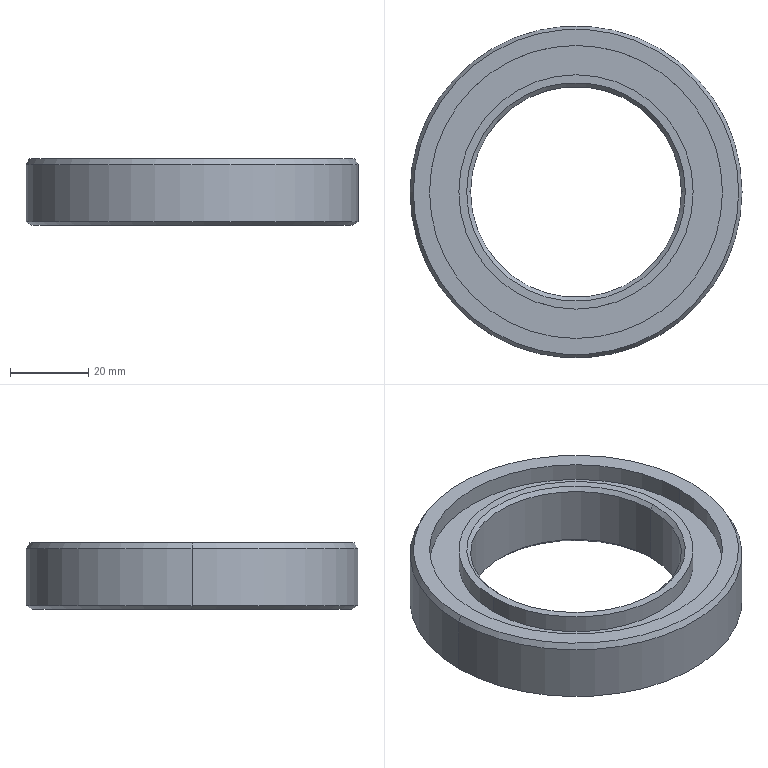Part | SolidWorks | features Chamfer 2, ICE 2, Extrusion 1 | 1 solid | 26 faces | box 85 x 85 x 17 mm | volume 42385 mm3 | cylinder 12 | cone 8 | plane 6 | commonest cylinder face diameters 60 x4 75 x4 54 x2 85 x2
STEP:
#1=CARTESIAN_POINT('',(-27.,0.,16.));
#2=VERTEX_POINT('',#1);
#3=CARTESIAN_POINT('',(27.,0.,16.));
#4=VERTEX_POINT('',#3);
#5=CARTESIAN_POINT('',(0.,0.,16.));
#6=DIRECTION('',(0.,0.,1.));
#7=DIRECTION('',(1.,0.,0.));
#8=AXIS2_PLACEMENT_3D('',#5,#6,#7);
#9=CIRCLE('',#8,27.);
#10=EDGE_CURVE('',#2,#4,#9,.T.);
#11=ORIENTED_EDGE('',*,*,#10,.F.);
#12=CARTESIAN_POINT('',(-28.,0.,17.));
#13=VERTEX_POINT('',#12);
#14=CARTESIAN_POINT('',(-27.,0.,16.));
#15=DIRECTION('',(-0.7071,0.,0.7071));
#16=VECTOR('',#15,1000.);
#17=LINE('',#14,#16);
#18=EDGE_CURVE('',#2,#13,#17,.T.);
#19=ORIENTED_EDGE('',*,*,#18,.T.);
#20=CARTESIAN_POINT('',(28.,0.,17.));
#21=VERTEX_POINT('',#20);
#22=CARTESIAN_POINT('',(0.,0.,17.));
#23=DIRECTION('',(0.,0.,-1.));
#24=DIRECTION('',(1.,0.,0.));
#25=AXIS2_PLACEMENT_3D('',#22,#23,#24);
#26=CIRCLE('',#25,28.);
#27=EDGE_CURVE('',#21,#13,#26,.T.);
#28=ORIENTED_EDGE('',*,*,#27,.F.);
#29=CARTESIAN_POINT('',(27.,0.,16.));
#30=DIRECTION('',(0.7071,0.,0.7071));
#31=VECTOR('',#30,1000.);
#32=LINE('',#29,#31);
#33=EDGE_CURVE('',#4,#21,#32,.T.);
#34=ORIENTED_EDGE('',*,*,#33,.F.);
#35=EDGE_LOOP('',(#11,#19,#28,#34));
#36=FACE_OUTER_BOUND('',#35,.T.);
#37=CARTESIAN_POINT('',(0.,0.,16.));
#38=DIRECTION('',(0.,0.,1.));
#39=DIRECTION('',(1.,0.,0.));
#40=AXIS2_PLACEMENT_3D('',#37,#38,#39);
#41=CONICAL_SURFACE('',#40,27.,0.7854);
#42=ADVANCED_FACE('',(#36),#41,.F.);
#43=CARTESIAN_POINT('',(27.,0.,1.));
#44=VERTEX_POINT('',#43);
#45=CARTESIAN_POINT('',(-27.,0.,1.));
#46=VERTEX_POINT('',#45);
#47=CARTESIAN_POINT('',(0.,0.,1.));
#48=DIRECTION('',(0.,0.,-1.));
#49=DIRECTION('',(1.,0.,0.));
#50=AXIS2_PLACEMENT_3D('',#47,#48,#49);
#51=CIRCLE('',#50,27.);
#52=EDGE_CURVE('',#44,#46,#51,.T.);
#53=ORIENTED_EDGE('',*,*,#52,.F.);
#54=CARTESIAN_POINT('',(28.,0.,0.));
#55=VERTEX_POINT('',#54);
#56=CARTESIAN_POINT('',(28.,0.,0.));
#57=DIRECTION('',(0.7071,0.,-0.7071));
#58=VECTOR('',#57,1000.);
#59=LINE('',#56,#58);
#60=EDGE_CURVE('',#44,#55,#59,.T.);
#61=ORIENTED_EDGE('',*,*,#60,.T.);
#62=CARTESIAN_POINT('',(-28.,0.,0.));
#63=VERTEX_POINT('',#62);
#64=CARTESIAN_POINT('',(0.,0.,0.));
#65=DIRECTION('',(0.,0.,1.));
#66=DIRECTION('',(1.,0.,0.));
#67=AXIS2_PLACEMENT_3D('',#64,#65,#66);
#68=CIRCLE('',#67,28.);
#69=EDGE_CURVE('',#63,#55,#68,.T.);
#70=ORIENTED_EDGE('',*,*,#69,.F.);
#71=CARTESIAN_POINT('',(-28.,0.,0.));
#72=DIRECTION('',(-0.7071,0.,-0.7071));
#73=VECTOR('',#72,1000.);
#74=LINE('',#71,#73);
#75=EDGE_CURVE('',#46,#63,#74,.T.);
#76=ORIENTED_EDGE('',*,*,#75,.F.);
#77=EDGE_LOOP('',(#53,#61,#70,#76));
#78=FACE_OUTER_BOUND('',#77,.T.);
#79=CARTESIAN_POINT('',(0.,0.,0.));
#80=DIRECTION('',(0.,0.,-1.));
#81=DIRECTION('',(-1.,0.,0.));
#82=AXIS2_PLACEMENT_3D('',#79,#80,#81);
#83=CONICAL_SURFACE('',#82,28.,0.7854);
#84=ADVANCED_FACE('',(#78),#83,.F.);
#85=CARTESIAN_POINT('',(-41.,0.,0.));
#86=VERTEX_POINT('',#85);
#87=CARTESIAN_POINT('',(41.,0.,0.));
#88=VERTEX_POINT('',#87);
#89=CARTESIAN_POINT('',(0.,0.,0.));
#90=DIRECTION('',(0.,0.,-1.));
#91=DIRECTION('',(1.,0.,0.));
#92=AXIS2_PLACEMENT_3D('',#89,#90,#91);
#93=CIRCLE('',#92,41.);
#94=EDGE_CURVE('',#86,#88,#93,.T.);
#95=ORIENTED_EDGE('',*,*,#94,.F.);
#96=CARTESIAN_POINT('',(-42.5,0.,0.866));
#97=VERTEX_POINT('',#96);
#98=CARTESIAN_POINT('',(-42.5,0.,0.866));
#99=DIRECTION('',(-0.866,0.,0.5));
#100=VECTOR('',#99,1000.);
#101=LINE('',#98,#100);
#102=EDGE_CURVE('',#86,#97,#101,.T.);
#103=ORIENTED_EDGE('',*,*,#102,.T.);
#104=CARTESIAN_POINT('',(42.5,0.,0.866));
#105=VERTEX_POINT('',#104);
#106=CARTESIAN_POINT('',(0.,0.,0.866));
#107=DIRECTION('',(0.,0.,1.));
#108=DIRECTION('',(1.,0.,0.));
#109=AXIS2_PLACEMENT_3D('',#106,#107,#108);
#110=CIRCLE('',#109,42.5);
#111=EDGE_CURVE('',#105,#97,#110,.T.);
#112=ORIENTED_EDGE('',*,*,#111,.F.);
#113=CARTESIAN_POINT('',(42.5,0.,0.866));
#114=DIRECTION('',(0.866,0.,0.5));
#115=VECTOR('',#114,1000.);
#116=LINE('',#113,#115);
#117=EDGE_CURVE('',#88,#105,#116,.T.);
#118=ORIENTED_EDGE('',*,*,#117,.F.);
#119=EDGE_LOOP('',(#95,#103,#112,#118));
#120=FACE_OUTER_BOUND('',#119,.T.);
#121=CARTESIAN_POINT('',(0.,0.,0.866));
#122=DIRECTION('',(0.,0.,1.));
#123=DIRECTION('',(1.,0.,0.));
#124=AXIS2_PLACEMENT_3D('',#121,#122,#123);
#125=CONICAL_SURFACE('',#124,42.5,1.047);
#126=ADVANCED_FACE('',(#120),#125,.T.);
#127=CARTESIAN_POINT('',(41.634,0.,17.));
#128=VERTEX_POINT('',#127);
#129=CARTESIAN_POINT('',(-41.634,0.,17.));
#130=VERTEX_POINT('',#129);
#131=CARTESIAN_POINT('',(0.,0.,17.));
#132=DIRECTION('',(0.,0.,1.));
#133=DIRECTION('',(1.,0.,0.));
#134=AXIS2_PLACEMENT_3D('',#131,#132,#133);
#135=CIRCLE('',#134,41.634);
#136=EDGE_CURVE('',#128,#130,#135,.T.);
#137=ORIENTED_EDGE('',*,*,#136,.F.);
#138=CARTESIAN_POINT('',(42.5,0.,15.5));
#139=VERTEX_POINT('',#138);
#140=CARTESIAN_POINT('',(41.634,0.,17.));
#141=DIRECTION('',(0.5,0.,-0.866));
#142=VECTOR('',#141,1000.);
#143=LINE('',#140,#142);
#144=EDGE_CURVE('',#128,#139,#143,.T.);
#145=ORIENTED_EDGE('',*,*,#144,.T.);
#146=CARTESIAN_POINT('',(-42.5,0.,15.5));
#147=VERTEX_POINT('',#146);
#148=CARTESIAN_POINT('',(0.,0.,15.5));
#149=DIRECTION('',(0.,0.,-1.));
#150=DIRECTION('',(1.,0.,0.));
#151=AXIS2_PLACEMENT_3D('',#148,#149,#150);
#152=CIRCLE('',#151,42.5);
#153=EDGE_CURVE('',#147,#139,#152,.T.);
#154=ORIENTED_EDGE('',*,*,#153,.F.);
#155=CARTESIAN_POINT('',(-41.634,0.,17.));
#156=DIRECTION('',(-0.5,0.,-0.866));
#157=VECTOR('',#156,1000.);
#158=LINE('',#155,#157);
#159=EDGE_CURVE('',#130,#147,#158,.T.);
#160=ORIENTED_EDGE('',*,*,#159,.F.);
#161=EDGE_LOOP('',(#137,#145,#154,#160));
#162=FACE_OUTER_BOUND('',#161,.T.);
#163=CARTESIAN_POINT('',(0.,0.,17.));
#164=DIRECTION('',(0.,0.,-1.));
#165=DIRECTION('',(-1.,0.,0.));
#166=AXIS2_PLACEMENT_3D('',#163,#164,#165);
#167=CONICAL_SURFACE('',#166,41.634,0.5236);
#168=ADVANCED_FACE('',(#162),#167,.T.);
#169=CARTESIAN_POINT('',(-30.,0.,4.6));
#170=VERTEX_POINT('',#169);
#171=CARTESIAN_POINT('',(30.,0.,4.6));
#172=VERTEX_POINT('',#171);
#173=CARTESIAN_POINT('',(0.,0.,4.6));
#174=DIRECTION('',(0.,0.,-1.));
#175=DIRECTION('',(-1.,0.,0.));
#176=AXIS2_PLACEMENT_3D('',#173,#174,#175);
#177=CIRCLE('',#176,30.);
#178=EDGE_CURVE('',#170,#172,#177,.T.);
#179=ORIENTED_EDGE('',*,*,#178,.T.);
#180=CARTESIAN_POINT('',(30.,0.,0.));
#181=VERTEX_POINT('',#180);
#182=CARTESIAN_POINT('',(30.,0.,4.6));
#183=DIRECTION('',(0.,0.,-1.));
#184=VECTOR('',#183,1000.);
#185=LINE('',#182,#184);
#186=EDGE_CURVE('',#172,#181,#185,.T.);
#187=ORIENTED_EDGE('',*,*,#186,.T.);
#188=CARTESIAN_POINT('',(-30.,0.,0.));
#189=VERTEX_POINT('',#188);
#190=CARTESIAN_POINT('',(0.,0.,0.));
#191=DIRECTION('',(0.,0.,-1.));
#192=DIRECTION('',(-1.,0.,0.));
#193=AXIS2_PLACEMENT_3D('',#190,#191,#192);
#194=CIRCLE('',#193,30.);
#195=EDGE_CURVE('',#189,#181,#194,.T.);
#196=ORIENTED_EDGE('',*,*,#195,.F.);
#197=CARTESIAN_POINT('',(-30.,0.,4.6));
#198=DIRECTION('',(0.,0.,-1.));
#199=VECTOR('',#198,1000.);
#200=LINE('',#197,#199);
#201=EDGE_CURVE('',#170,#189,#200,.T.);
#202=ORIENTED_EDGE('',*,*,#201,.F.);
#203=EDGE_LOOP('',(#179,#187,#196,#202));
#204=FACE_OUTER_BOUND('',#203,.T.);
#205=CARTESIAN_POINT('',(0.,0.,4.6));
#206=DIRECTION('',(0.,0.,-1.));
#207=DIRECTION('',(-1.,0.,0.));
#208=AXIS2_PLACEMENT_3D('',#205,#206,#207);
#209=CYLINDRICAL_SURFACE('',#208,30.);
#210=ADVANCED_FACE('',(#204),#209,.T.);
#211=CARTESIAN_POINT('',(37.5,0.,4.6));
#212=VERTEX_POINT('',#211);
#213=CARTESIAN_POINT('',(-37.5,0.,4.6));
#214=VERTEX_POINT('',#213);
#215=CARTESIAN_POINT('',(0.,0.,4.6));
#216=DIRECTION('',(0.,0.,-1.));
#217=DIRECTION('',(-1.,0.,0.));
#218=AXIS2_PLACEMENT_3D('',#215,#216,#217);
#219=CIRCLE('',#218,37.5);
#220=EDGE_CURVE('',#212,#214,#219,.T.);
#221=ORIENTED_EDGE('',*,*,#220,.F.);
#222=CARTESIAN_POINT('',(37.5,0.,0.));
#223=VERTEX_POINT('',#222);
#224=CARTESIAN_POINT('',(37.5,0.,4.6));
#225=DIRECTION('',(0.,0.,-1.));
#226=VECTOR('',#225,1000.);
#227=LINE('',#224,#226);
#228=EDGE_CURVE('',#212,#223,#227,.T.);
#229=ORIENTED_EDGE('',*,*,#228,.T.);
#230=CARTESIAN_POINT('',(-37.5,0.,0.));
#231=VERTEX_POINT('',#230);
#232=CARTESIAN_POINT('',(0.,0.,0.));
#233=DIRECTION('',(0.,0.,-1.));
#234=DIRECTION('',(-1.,0.,0.));
#235=AXIS2_PLACEMENT_3D('',#232,#233,#234);
#236=CIRCLE('',#235,37.5);
#237=EDGE_CURVE('',#223,#231,#236,.T.);
#238=ORIENTED_EDGE('',*,*,#237,.T.);
#239=CARTESIAN_POINT('',(-37.5,0.,4.6));
#240=DIRECTION('',(0.,0.,-1.));
#241=VECTOR('',#240,1000.);
#242=LINE('',#239,#241);
#243=EDGE_CURVE('',#214,#231,#242,.T.);
#244=ORIENTED_EDGE('',*,*,#243,.F.);
#245=EDGE_LOOP('',(#221,#229,#238,#244));
#246=FACE_OUTER_BOUND('',#245,.T.);
#247=CARTESIAN_POINT('',(0.,0.,4.6));
#248=DIRECTION('',(0.,0.,-1.));
#249=DIRECTION('',(-1.,0.,0.));
#250=AXIS2_PLACEMENT_3D('',#247,#248,#249);
#251=CYLINDRICAL_SURFACE('',#250,37.5);
#252=ADVANCED_FACE('',(#246),#251,.F.);
#253=CARTESIAN_POINT('',(30.,0.,12.4));
#254=VERTEX_POINT('',#253);
#255=CARTESIAN_POINT('',(-30.,0.,12.4));
#256=VERTEX_POINT('',#255);
#257=CARTESIAN_POINT('',(0.,0.,12.4));
#258=DIRECTION('',(0.,0.,1.));
#259=DIRECTION('',(1.,0.,0.));
#260=AXIS2_PLACEMENT_3D('',#257,#258,#259);
#261=CIRCLE('',#260,30.);
#262=EDGE_CURVE('',#254,#256,#261,.T.);
#263=ORIENTED_EDGE('',*,*,#262,.T.);
#264=CARTESIAN_POINT('',(-30.,0.,17.));
#265=VERTEX_POINT('',#264);
#266=CARTESIAN_POINT('',(-30.,0.,12.4));
#267=DIRECTION('',(0.,0.,1.));
#268=VECTOR('',#267,1000.);
#269=LINE('',#266,#268);
#270=EDGE_CURVE('',#256,#265,#269,.T.);
#271=ORIENTED_EDGE('',*,*,#270,.T.);
#272=CARTESIAN_POINT('',(30.,0.,17.));
#273=VERTEX_POINT('',#272);
#274=CARTESIAN_POINT('',(0.,0.,17.));
#275=DIRECTION('',(0.,0.,1.));
#276=DIRECTION('',(1.,0.,0.));
#277=AXIS2_PLACEMENT_3D('',#274,#275,#276);
#278=CIRCLE('',#277,30.);
#279=EDGE_CURVE('',#273,#265,#278,.T.);
#280=ORIENTED_EDGE('',*,*,#279,.F.);
#281=CARTESIAN_POINT('',(30.,0.,12.4));
#282=DIRECTION('',(0.,0.,1.));
#283=VECTOR('',#282,1000.);
#284=LINE('',#281,#283);
#285=EDGE_CURVE('',#254,#273,#284,.T.);
#286=ORIENTED_EDGE('',*,*,#285,.F.);
#287=EDGE_LOOP('',(#263,#271,#280,#286));
#288=FACE_OUTER_BOUND('',#287,.T.);
#289=CARTESIAN_POINT('',(0.,0.,12.4));
#290=DIRECTION('',(0.,0.,1.));
#291=DIRECTION('',(1.,0.,0.));
#292=AXIS2_PLACEMENT_3D('',#289,#290,#291);
#293=CYLINDRICAL_SURFACE('',#292,30.);
#294=ADVANCED_FACE('',(#288),#293,.T.);
#295=CARTESIAN_POINT('',(-37.5,0.,12.4));
#296=VERTEX_POINT('',#295);
#297=CARTESIAN_POINT('',(37.5,0.,12.4));
#298=VERTEX_POINT('',#297);
#299=CARTESIAN_POINT('',(0.,0.,12.4));
#300=DIRECTION('',(0.,0.,1.));
#301=DIRECTION('',(1.,0.,0.));
#302=AXIS2_PLACEMENT_3D('',#299,#300,#301);
#303=CIRCLE('',#302,37.5);
#304=EDGE_CURVE('',#296,#298,#303,.T.);
#305=ORIENTED_EDGE('',*,*,#304,.F.);
#306=CARTESIAN_POINT('',(-37.5,0.,17.));
#307=VERTEX_POINT('',#306);
#308=CARTESIAN_POINT('',(-37.5,0.,12.4));
#309=DIRECTION('',(0.,0.,1.));
#310=VECTOR('',#309,1000.);
#311=LINE('',#308,#310);
#312=EDGE_CURVE('',#296,#307,#311,.T.);
#313=ORIENTED_EDGE('',*,*,#312,.T.);
#314=CARTESIAN_POINT('',(37.5,0.,17.));
#315=VERTEX_POINT('',#314);
#316=CARTESIAN_POINT('',(0.,0.,17.));
#317=DIRECTION('',(0.,0.,1.));
#318=DIRECTION('',(1.,0.,0.));
#319=AXIS2_PLACEMENT_3D('',#316,#317,#318);
#320=CIRCLE('',#319,37.5);
#321=EDGE_CURVE('',#307,#315,#320,.T.);
#322=ORIENTED_EDGE('',*,*,#321,.T.);
#323=CARTESIAN_POINT('',(37.5,0.,12.4));
#324=DIRECTION('',(0.,0.,1.));
#325=VECTOR('',#324,1000.);
#326=LINE('',#323,#325);
#327=EDGE_CURVE('',#298,#315,#326,.T.);
#328=ORIENTED_EDGE('',*,*,#327,.F.);
#329=EDGE_LOOP('',(#305,#313,#322,#328));
#330=FACE_OUTER_BOUND('',#329,.T.);
#331=CARTESIAN_POINT('',(0.,0.,12.4));
#332=DIRECTION('',(0.,0.,1.));
#333=DIRECTION('',(1.,0.,0.));
#334=AXIS2_PLACEMENT_3D('',#331,#332,#333);
#335=CYLINDRICAL_SURFACE('',#334,37.5);
#336=ADVANCED_FACE('',(#330),#335,.F.);
#337=ORIENTED_EDGE('',*,*,#10,.T.);
#338=CARTESIAN_POINT('',(27.,0.,17.));
#339=DIRECTION('',(0.,0.,-1.));
#340=VECTOR('',#339,1000.);
#341=LINE('',#338,#340);
#342=EDGE_CURVE('',#4,#44,#341,.T.);
#343=ORIENTED_EDGE('',*,*,#342,.T.);
#344=ORIENTED_EDGE('',*,*,#52,.T.);
#345=CARTESIAN_POINT('',(-27.,0.,17.));
#346=DIRECTION('',(0.,0.,-1.));
#347=VECTOR('',#346,1000.);
#348=LINE('',#345,#347);
#349=EDGE_CURVE('',#2,#46,#348,.T.);
#350=ORIENTED_EDGE('',*,*,#349,.F.);
#351=EDGE_LOOP('',(#337,#343,#344,#350));
#352=FACE_OUTER_BOUND('',#351,.T.);
#353=CARTESIAN_POINT('',(0.,0.,17.));
#354=DIRECTION('',(0.,0.,-1.));
#355=DIRECTION('',(-1.,0.,0.));
#356=AXIS2_PLACEMENT_3D('',#353,#354,#355);
#357=CYLINDRICAL_SURFACE('',#356,27.);
#358=ADVANCED_FACE('',(#352),#357,.F.);
#359=ORIENTED_EDGE('',*,*,#153,.T.);
#360=CARTESIAN_POINT('',(42.5,0.,17.));
#361=DIRECTION('',(0.,0.,-1.));
#362=VECTOR('',#361,1000.);
#363=LINE('',#360,#362);
#364=EDGE_CURVE('',#139,#105,#363,.T.);
#365=ORIENTED_EDGE('',*,*,#364,.T.);
#366=ORIENTED_EDGE('',*,*,#111,.T.);
#367=CARTESIAN_POINT('',(-42.5,0.,17.));
#368=DIRECTION('',(0.,0.,-1.));
#369=VECTOR('',#368,1000.);
#370=LINE('',#367,#369);
#371=EDGE_CURVE('',#147,#97,#370,.T.);
#372=ORIENTED_EDGE('',*,*,#371,.F.);
#373=EDGE_LOOP('',(#359,#365,#366,#372));
#374=FACE_OUTER_BOUND('',#373,.T.);
#375=CARTESIAN_POINT('',(0.,0.,17.));
#376=DIRECTION('',(0.,0.,-1.));
#377=DIRECTION('',(-1.,0.,0.));
#378=AXIS2_PLACEMENT_3D('',#375,#376,#377);
#379=CYLINDRICAL_SURFACE('',#378,42.5);
#380=ADVANCED_FACE('',(#374),#379,.T.);
#381=ORIENTED_EDGE('',*,*,#69,.T.);
#382=CARTESIAN_POINT('',(0.,0.,0.));
#383=DIRECTION('',(0.,0.,1.));
#384=DIRECTION('',(1.,0.,0.));
#385=AXIS2_PLACEMENT_3D('',#382,#383,#384);
#386=CIRCLE('',#385,28.);
#387=EDGE_CURVE('',#55,#63,#386,.T.);
#388=ORIENTED_EDGE('',*,*,#387,.T.);
#389=EDGE_LOOP('',(#381,#388));
#390=FACE_BOUND('',#389,.T.);
#391=ORIENTED_EDGE('',*,*,#195,.T.);
#392=CARTESIAN_POINT('',(0.,0.,0.));
#393=DIRECTION('',(0.,0.,-1.));
#394=DIRECTION('',(-1.,0.,0.));
#395=AXIS2_PLACEMENT_3D('',#392,#393,#394);
#396=CIRCLE('',#395,30.);
#397=EDGE_CURVE('',#181,#189,#396,.T.);
#398=ORIENTED_EDGE('',*,*,#397,.T.);
#399=EDGE_LOOP('',(#391,#398));
#400=FACE_OUTER_BOUND('',#399,.T.);
#401=CARTESIAN_POINT('',(0.,0.,0.));
#402=DIRECTION('',(0.,0.,1.));
#403=DIRECTION('',(1.,0.,0.));
#404=AXIS2_PLACEMENT_3D('',#401,#402,#403);
#405=PLANE('',#404);
#406=ADVANCED_FACE('',(#390,#400),#405,.F.);
#407=ORIENTED_EDGE('',*,*,#27,.T.);
#408=CARTESIAN_POINT('',(0.,0.,17.));
#409=DIRECTION('',(0.,0.,-1.));
#410=DIRECTION('',(1.,0.,0.));
#411=AXIS2_PLACEMENT_3D('',#408,#409,#410);
#412=CIRCLE('',#411,28.);
#413=EDGE_CURVE('',#13,#21,#412,.T.);
#414=ORIENTED_EDGE('',*,*,#413,.T.);
#415=EDGE_LOOP('',(#407,#414));
#416=FACE_BOUND('',#415,.T.);
#417=ORIENTED_EDGE('',*,*,#279,.T.);
#418=CARTESIAN_POINT('',(0.,0.,17.));
#419=DIRECTION('',(0.,0.,1.));
#420=DIRECTION('',(1.,0.,0.));
#421=AXIS2_PLACEMENT_3D('',#418,#419,#420);
#422=CIRCLE('',#421,30.);
#423=EDGE_CURVE('',#265,#273,#422,.T.);
#424=ORIENTED_EDGE('',*,*,#423,.T.);
#425=EDGE_LOOP('',(#417,#424));
#426=FACE_OUTER_BOUND('',#425,.T.);
#427=CARTESIAN_POINT('',(0.,0.,17.));
#428=DIRECTION('',(0.,0.,1.));
#429=DIRECTION('',(1.,0.,0.));
#430=AXIS2_PLACEMENT_3D('',#427,#428,#429);
#431=PLANE('',#430);
#432=ADVANCED_FACE('',(#416,#426),#431,.T.);
#433=CARTESIAN_POINT('',(0.,0.,17.));
#434=DIRECTION('',(0.,0.,1.));
#435=DIRECTION('',(1.,0.,0.));
#436=AXIS2_PLACEMENT_3D('',#433,#434,#435);
#437=CIRCLE('',#436,41.634);
#438=EDGE_CURVE('',#130,#128,#437,.T.);
#439=ORIENTED_EDGE('',*,*,#438,.T.);
#440=ORIENTED_EDGE('',*,*,#136,.T.);
#441=EDGE_LOOP('',(#439,#440));
#442=FACE_OUTER_BOUND('',#441,.T.);
#443=CARTESIAN_POINT('',(0.,0.,17.));
#444=DIRECTION('',(0.,0.,1.));
#445=DIRECTION('',(1.,0.,0.));
#446=AXIS2_PLACEMENT_3D('',#443,#444,#445);
#447=CIRCLE('',#446,37.5);
#448=EDGE_CURVE('',#315,#307,#447,.T.);
#449=ORIENTED_EDGE('',*,*,#448,.F.);
#450=ORIENTED_EDGE('',*,*,#321,.F.);
#451=EDGE_LOOP('',(#449,#450));
#452=FACE_BOUND('',#451,.T.);
#453=CARTESIAN_POINT('',(0.,0.,17.));
#454=DIRECTION('',(0.,0.,1.));
#455=DIRECTION('',(1.,0.,0.));
#456=AXIS2_PLACEMENT_3D('',#453,#454,#455);
#457=PLANE('',#456);
#458=ADVANCED_FACE('',(#442,#452),#457,.T.);
#459=CARTESIAN_POINT('',(0.,0.,0.));
#460=DIRECTION('',(0.,0.,-1.));
#461=DIRECTION('',(1.,0.,0.));
#462=AXIS2_PLACEMENT_3D('',#459,#460,#461);
#463=CIRCLE('',#462,41.);
#464=EDGE_CURVE('',#88,#86,#463,.T.);
#465=ORIENTED_EDGE('',*,*,#464,.T.);
#466=ORIENTED_EDGE('',*,*,#94,.T.);
#467=EDGE_LOOP('',(#465,#466));
#468=FACE_OUTER_BOUND('',#467,.T.);
#469=CARTESIAN_POINT('',(0.,0.,0.));
#470=DIRECTION('',(0.,0.,-1.));
#471=DIRECTION('',(-1.,0.,0.));
#472=AXIS2_PLACEMENT_3D('',#469,#470,#471);
#473=CIRCLE('',#472,37.5);
#474=EDGE_CURVE('',#231,#223,#473,.T.);
#475=ORIENTED_EDGE('',*,*,#474,.F.);
#476=ORIENTED_EDGE('',*,*,#237,.F.);
#477=EDGE_LOOP('',(#475,#476));
#478=FACE_BOUND('',#477,.T.);
#479=CARTESIAN_POINT('',(0.,0.,0.));
#480=DIRECTION('',(0.,0.,1.));
#481=DIRECTION('',(1.,0.,0.));
#482=AXIS2_PLACEMENT_3D('',#479,#480,#481);
#483=PLANE('',#482);
#484=ADVANCED_FACE('',(#468,#478),#483,.F.);
#485=ORIENTED_EDGE('',*,*,#364,.F.);
#486=CARTESIAN_POINT('',(0.,0.,15.5));
#487=DIRECTION('',(0.,0.,-1.));
#488=DIRECTION('',(1.,0.,0.));
#489=AXIS2_PLACEMENT_3D('',#486,#487,#488);
#490=CIRCLE('',#489,42.5);
#491=EDGE_CURVE('',#139,#147,#490,.T.);
#492=ORIENTED_EDGE('',*,*,#491,.T.);
#493=ORIENTED_EDGE('',*,*,#371,.T.);
#494=CARTESIAN_POINT('',(0.,0.,0.866));
#495=DIRECTION('',(0.,0.,1.));
#496=DIRECTION('',(1.,0.,0.));
#497=AXIS2_PLACEMENT_3D('',#494,#495,#496);
#498=CIRCLE('',#497,42.5);
#499=EDGE_CURVE('',#97,#105,#498,.T.);
#500=ORIENTED_EDGE('',*,*,#499,.T.);
#501=EDGE_LOOP('',(#485,#492,#493,#500));
#502=FACE_OUTER_BOUND('',#501,.T.);
#503=CARTESIAN_POINT('',(0.,0.,17.));
#504=DIRECTION('',(0.,0.,-1.));
#505=DIRECTION('',(-1.,0.,0.));
#506=AXIS2_PLACEMENT_3D('',#503,#504,#505);
#507=CYLINDRICAL_SURFACE('',#506,42.5);
#508=ADVANCED_FACE('',(#502),#507,.T.);
#509=ORIENTED_EDGE('',*,*,#342,.F.);
#510=CARTESIAN_POINT('',(0.,0.,16.));
#511=DIRECTION('',(0.,0.,1.));
#512=DIRECTION('',(1.,0.,0.));
#513=AXIS2_PLACEMENT_3D('',#510,#511,#512);
#514=CIRCLE('',#513,27.);
#515=EDGE_CURVE('',#4,#2,#514,.T.);
#516=ORIENTED_EDGE('',*,*,#515,.T.);
#517=ORIENTED_EDGE('',*,*,#349,.T.);
#518=CARTESIAN_POINT('',(0.,0.,1.));
#519=DIRECTION('',(0.,0.,-1.));
#520=DIRECTION('',(1.,0.,0.));
#521=AXIS2_PLACEMENT_3D('',#518,#519,#520);
#522=CIRCLE('',#521,27.);
#523=EDGE_CURVE('',#46,#44,#522,.T.);
#524=ORIENTED_EDGE('',*,*,#523,.T.);
#525=EDGE_LOOP('',(#509,#516,#517,#524));
#526=FACE_OUTER_BOUND('',#525,.T.);
#527=CARTESIAN_POINT('',(0.,0.,17.));
#528=DIRECTION('',(0.,0.,-1.));
#529=DIRECTION('',(-1.,0.,0.));
#530=AXIS2_PLACEMENT_3D('',#527,#528,#529);
#531=CYLINDRICAL_SURFACE('',#530,27.);
#532=ADVANCED_FACE('',(#526),#531,.F.);
#533=ORIENTED_EDGE('',*,*,#312,.F.);
#534=CARTESIAN_POINT('',(0.,0.,12.4));
#535=DIRECTION('',(0.,0.,1.));
#536=DIRECTION('',(1.,0.,0.));
#537=AXIS2_PLACEMENT_3D('',#534,#535,#536);
#538=CIRCLE('',#537,37.5);
#539=EDGE_CURVE('',#298,#296,#538,.T.);
#540=ORIENTED_EDGE('',*,*,#539,.F.);
#541=ORIENTED_EDGE('',*,*,#327,.T.);
#542=ORIENTED_EDGE('',*,*,#448,.T.);
#543=EDGE_LOOP('',(#533,#540,#541,#542));
#544=FACE_OUTER_BOUND('',#543,.T.);
#545=CARTESIAN_POINT('',(0.,0.,12.4));
#546=DIRECTION('',(0.,0.,1.));
#547=DIRECTION('',(1.,0.,0.));
#548=AXIS2_PLACEMENT_3D('',#545,#546,#547);
#549=CYLINDRICAL_SURFACE('',#548,37.5);
#550=ADVANCED_FACE('',(#544),#549,.F.);
#551=ORIENTED_EDGE('',*,*,#262,.F.);
#552=CARTESIAN_POINT('',(0.,0.,12.4));
#553=DIRECTION('',(0.,0.,1.));
#554=DIRECTION('',(1.,0.,0.));
#555=AXIS2_PLACEMENT_3D('',#552,#553,#554);
#556=CIRCLE('',#555,30.);
#557=EDGE_CURVE('',#256,#254,#556,.T.);
#558=ORIENTED_EDGE('',*,*,#557,.F.);
#559=EDGE_LOOP('',(#551,#558));
#560=FACE_BOUND('',#559,.T.);
#561=ORIENTED_EDGE('',*,*,#539,.T.);
#562=ORIENTED_EDGE('',*,*,#304,.T.);
#563=EDGE_LOOP('',(#561,#562));
#564=FACE_OUTER_BOUND('',#563,.T.);
#565=CARTESIAN_POINT('',(0.,0.,12.4));
#566=DIRECTION('',(0.,0.,1.));
#567=DIRECTION('',(1.,0.,0.));
#568=AXIS2_PLACEMENT_3D('',#565,#566,#567);
#569=PLANE('',#568);
#570=ADVANCED_FACE('',(#560,#564),#569,.T.);
#571=ORIENTED_EDGE('',*,*,#270,.F.);
#572=ORIENTED_EDGE('',*,*,#557,.T.);
#573=ORIENTED_EDGE('',*,*,#285,.T.);
#574=ORIENTED_EDGE('',*,*,#423,.F.);
#575=EDGE_LOOP('',(#571,#572,#573,#574));
#576=FACE_OUTER_BOUND('',#575,.T.);
#577=CARTESIAN_POINT('',(0.,0.,12.4));
#578=DIRECTION('',(0.,0.,1.));
#579=DIRECTION('',(1.,0.,0.));
#580=AXIS2_PLACEMENT_3D('',#577,#578,#579);
#581=CYLINDRICAL_SURFACE('',#580,30.);
#582=ADVANCED_FACE('',(#576),#581,.T.);
#583=ORIENTED_EDGE('',*,*,#228,.F.);
#584=CARTESIAN_POINT('',(0.,0.,4.6));
#585=DIRECTION('',(0.,0.,-1.));
#586=DIRECTION('',(-1.,0.,0.));
#587=AXIS2_PLACEMENT_3D('',#584,#585,#586);
#588=CIRCLE('',#587,37.5);
#589=EDGE_CURVE('',#214,#212,#588,.T.);
#590=ORIENTED_EDGE('',*,*,#589,.F.);
#591=ORIENTED_EDGE('',*,*,#243,.T.);
#592=ORIENTED_EDGE('',*,*,#474,.T.);
#593=EDGE_LOOP('',(#583,#590,#591,#592));
#594=FACE_OUTER_BOUND('',#593,.T.);
#595=CARTESIAN_POINT('',(0.,0.,4.6));
#596=DIRECTION('',(0.,0.,-1.));
#597=DIRECTION('',(-1.,0.,0.));
#598=AXIS2_PLACEMENT_3D('',#595,#596,#597);
#599=CYLINDRICAL_SURFACE('',#598,37.5);
#600=ADVANCED_FACE('',(#594),#599,.F.);
#601=ORIENTED_EDGE('',*,*,#178,.F.);
#602=CARTESIAN_POINT('',(0.,0.,4.6));
#603=DIRECTION('',(0.,0.,-1.));
#604=DIRECTION('',(-1.,0.,0.));
#605=AXIS2_PLACEMENT_3D('',#602,#603,#604);
#606=CIRCLE('',#605,30.);
#607=EDGE_CURVE('',#172,#170,#606,.T.);
#608=ORIENTED_EDGE('',*,*,#607,.F.);
#609=EDGE_LOOP('',(#601,#608));
#610=FACE_BOUND('',#609,.T.);
#611=ORIENTED_EDGE('',*,*,#589,.T.);
#612=ORIENTED_EDGE('',*,*,#220,.T.);
#613=EDGE_LOOP('',(#611,#612));
#614=FACE_OUTER_BOUND('',#613,.T.);
#615=CARTESIAN_POINT('',(0.,0.,4.6));
#616=DIRECTION('',(0.,0.,-1.));
#617=DIRECTION('',(-1.,0.,0.));
#618=AXIS2_PLACEMENT_3D('',#615,#616,#617);
#619=PLANE('',#618);
#620=ADVANCED_FACE('',(#610,#614),#619,.T.);
#621=ORIENTED_EDGE('',*,*,#186,.F.);
#622=ORIENTED_EDGE('',*,*,#607,.T.);
#623=ORIENTED_EDGE('',*,*,#201,.T.);
#624=ORIENTED_EDGE('',*,*,#397,.F.);
#625=EDGE_LOOP('',(#621,#622,#623,#624));
#626=FACE_OUTER_BOUND('',#625,.T.);
#627=CARTESIAN_POINT('',(0.,0.,4.6));
#628=DIRECTION('',(0.,0.,-1.));
#629=DIRECTION('',(-1.,0.,0.));
#630=AXIS2_PLACEMENT_3D('',#627,#628,#629);
#631=CYLINDRICAL_SURFACE('',#630,30.);
#632=ADVANCED_FACE('',(#626),#631,.T.);
#633=ORIENTED_EDGE('',*,*,#144,.F.);
#634=ORIENTED_EDGE('',*,*,#438,.F.);
#635=ORIENTED_EDGE('',*,*,#159,.T.);
#636=ORIENTED_EDGE('',*,*,#491,.F.);
#637=EDGE_LOOP('',(#633,#634,#635,#636));
#638=FACE_OUTER_BOUND('',#637,.T.);
#639=CARTESIAN_POINT('',(0.,0.,17.));
#640=DIRECTION('',(0.,0.,-1.));
#641=DIRECTION('',(-1.,0.,0.));
#642=AXIS2_PLACEMENT_3D('',#639,#640,#641);
#643=CONICAL_SURFACE('',#642,41.634,0.5236);
#644=ADVANCED_FACE('',(#638),#643,.T.);
#645=ORIENTED_EDGE('',*,*,#102,.F.);
#646=ORIENTED_EDGE('',*,*,#464,.F.);
#647=ORIENTED_EDGE('',*,*,#117,.T.);
#648=ORIENTED_EDGE('',*,*,#499,.F.);
#649=EDGE_LOOP('',(#645,#646,#647,#648));
#650=FACE_OUTER_BOUND('',#649,.T.);
#651=CARTESIAN_POINT('',(0.,0.,0.866));
#652=DIRECTION('',(0.,0.,1.));
#653=DIRECTION('',(1.,0.,0.));
#654=AXIS2_PLACEMENT_3D('',#651,#652,#653);
#655=CONICAL_SURFACE('',#654,42.5,1.047);
#656=ADVANCED_FACE('',(#650),#655,.T.);
#657=ORIENTED_EDGE('',*,*,#60,.F.);
#658=ORIENTED_EDGE('',*,*,#523,.F.);
#659=ORIENTED_EDGE('',*,*,#75,.T.);
#660=ORIENTED_EDGE('',*,*,#387,.F.);
#661=EDGE_LOOP('',(#657,#658,#659,#660));
#662=FACE_OUTER_BOUND('',#661,.T.);
#663=CARTESIAN_POINT('',(0.,0.,0.));
#664=DIRECTION('',(0.,0.,-1.));
#665=DIRECTION('',(-1.,0.,0.));
#666=AXIS2_PLACEMENT_3D('',#663,#664,#665);
#667=CONICAL_SURFACE('',#666,28.,0.7854);
#668=ADVANCED_FACE('',(#662),#667,.F.);
#669=ORIENTED_EDGE('',*,*,#18,.F.);
#670=ORIENTED_EDGE('',*,*,#515,.F.);
#671=ORIENTED_EDGE('',*,*,#33,.T.);
#672=ORIENTED_EDGE('',*,*,#413,.F.);
#673=EDGE_LOOP('',(#669,#670,#671,#672));
#674=FACE_OUTER_BOUND('',#673,.T.);
#675=CARTESIAN_POINT('',(0.,0.,16.));
#676=DIRECTION('',(0.,0.,1.));
#677=DIRECTION('',(1.,0.,0.));
#678=AXIS2_PLACEMENT_3D('',#675,#676,#677);
#679=CONICAL_SURFACE('',#678,27.,0.7854);
#680=ADVANCED_FACE('',(#674),#679,.F.);
#681=CLOSED_SHELL('',(#42,#84,#126,#168,#210,#252,#294,#336,#358,#380,#406,#432,#458,#484,#508,#532,#550,#570,#582,#600,#620,#632,#644,#656,#668,#680));
#682=MANIFOLD_SOLID_BREP('',#681);
#683=CARTESIAN_POINT('',(0.,0.,0.));
#684=DIRECTION('',(0.,0.,1.));
#685=DIRECTION('',(1.,0.,0.));
#686=AXIS2_PLACEMENT_3D('',#683,#684,#685);
#687=(LENGTH_UNIT()NAMED_UNIT(*)SI_UNIT(.MILLI.,.METRE.));
#688=UNCERTAINTY_MEASURE_WITH_UNIT(LENGTH_MEASURE(0.00001),#687,'','');
#689=(NAMED_UNIT(*)PLANE_ANGLE_UNIT()SI_UNIT($,.RADIAN.));
#690=(NAMED_UNIT(*)SI_UNIT($,.STERADIAN.)SOLID_ANGLE_UNIT());
#691=(GEOMETRIC_REPRESENTATION_CONTEXT(3)GLOBAL_UNCERTAINTY_ASSIGNED_CONTEXT((#688))GLOBAL_UNIT_ASSIGNED_CONTEXT((#687,#689,#690))REPRESENTATION_CONTEXT('',''));
#692=ADVANCED_BREP_SHAPE_REPRESENTATION('',(#682,#686),#691);